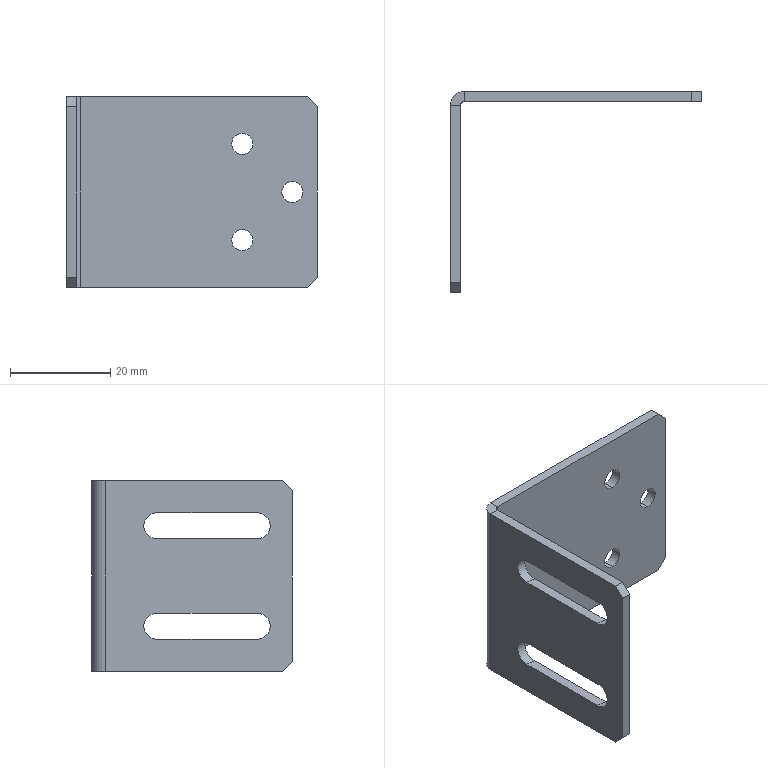Part | SolidWorks | features Chamfer 1, Cut 1, FlatPattern 1, HoleWzd 1, SMBaseFlange 1, SheetMetal 1 | 1 solid | 32 faces | box 50 x 40 x 38 mm | volume 6031 mm3 | plane 20 | cylinder 12 | commonest cylinder face diameters 4.2 x6 5.2 x4 1.473 x1 5.473 x1
STEP:
#1=CARTESIAN_POINT('',(35.,38.,7.5));
#2=VERTEX_POINT('',#1);
#3=CARTESIAN_POINT('',(35.,38.,11.7));
#4=VERTEX_POINT('',#3);
#5=CARTESIAN_POINT('',(35.,38.,9.6));
#6=DIRECTION('',(0.,1.,0.));
#7=DIRECTION('',(0.,0.,1.));
#8=AXIS2_PLACEMENT_3D('',#5,#6,#7);
#9=CIRCLE('',#8,2.1);
#10=EDGE_CURVE('',#2,#4,#9,.T.);
#11=ORIENTED_EDGE('',*,*,#10,.F.);
#12=CARTESIAN_POINT('',(35.,40.,7.5));
#13=VERTEX_POINT('',#12);
#14=CARTESIAN_POINT('',(35.,40.,7.5));
#15=DIRECTION('',(0.,1.,0.));
#16=VECTOR('',#15,1000.);
#17=LINE('',#14,#16);
#18=EDGE_CURVE('',#2,#13,#17,.T.);
#19=ORIENTED_EDGE('',*,*,#18,.T.);
#20=CARTESIAN_POINT('',(35.,40.,11.7));
#21=VERTEX_POINT('',#20);
#22=CARTESIAN_POINT('',(35.,40.,9.6));
#23=DIRECTION('',(0.,1.,0.));
#24=DIRECTION('',(0.,0.,1.));
#25=AXIS2_PLACEMENT_3D('',#22,#23,#24);
#26=CIRCLE('',#25,2.1);
#27=EDGE_CURVE('',#13,#21,#26,.T.);
#28=ORIENTED_EDGE('',*,*,#27,.T.);
#29=CARTESIAN_POINT('',(35.,40.,11.7));
#30=DIRECTION('',(0.,1.,0.));
#31=VECTOR('',#30,1000.);
#32=LINE('',#29,#31);
#33=EDGE_CURVE('',#4,#21,#32,.T.);
#34=ORIENTED_EDGE('',*,*,#33,.F.);
#35=EDGE_LOOP('',(#11,#19,#28,#34));
#36=FACE_OUTER_BOUND('',#35,.T.);
#37=CARTESIAN_POINT('',(35.,40.,9.6));
#38=DIRECTION('',(0.,1.,0.));
#39=DIRECTION('',(0.,0.,1.));
#40=AXIS2_PLACEMENT_3D('',#37,#38,#39);
#41=CYLINDRICAL_SURFACE('',#40,2.1);
#42=ADVANCED_FACE('',(#36),#41,.F.);
#43=CARTESIAN_POINT('',(45.,38.,-2.1));
#44=VERTEX_POINT('',#43);
#45=CARTESIAN_POINT('',(45.,38.,2.1));
#46=VERTEX_POINT('',#45);
#47=CARTESIAN_POINT('',(45.,38.,0.));
#48=DIRECTION('',(0.,1.,0.));
#49=DIRECTION('',(0.,0.,1.));
#50=AXIS2_PLACEMENT_3D('',#47,#48,#49);
#51=CIRCLE('',#50,2.1);
#52=EDGE_CURVE('',#44,#46,#51,.T.);
#53=ORIENTED_EDGE('',*,*,#52,.F.);
#54=CARTESIAN_POINT('',(45.,40.,-2.1));
#55=VERTEX_POINT('',#54);
#56=CARTESIAN_POINT('',(45.,40.,-2.1));
#57=DIRECTION('',(0.,1.,0.));
#58=VECTOR('',#57,1000.);
#59=LINE('',#56,#58);
#60=EDGE_CURVE('',#44,#55,#59,.T.);
#61=ORIENTED_EDGE('',*,*,#60,.T.);
#62=CARTESIAN_POINT('',(45.,40.,2.1));
#63=VERTEX_POINT('',#62);
#64=CARTESIAN_POINT('',(45.,40.,0.));
#65=DIRECTION('',(0.,1.,0.));
#66=DIRECTION('',(0.,0.,1.));
#67=AXIS2_PLACEMENT_3D('',#64,#65,#66);
#68=CIRCLE('',#67,2.1);
#69=EDGE_CURVE('',#55,#63,#68,.T.);
#70=ORIENTED_EDGE('',*,*,#69,.T.);
#71=CARTESIAN_POINT('',(45.,40.,2.1));
#72=DIRECTION('',(0.,1.,0.));
#73=VECTOR('',#72,1000.);
#74=LINE('',#71,#73);
#75=EDGE_CURVE('',#46,#63,#74,.T.);
#76=ORIENTED_EDGE('',*,*,#75,.F.);
#77=EDGE_LOOP('',(#53,#61,#70,#76));
#78=FACE_OUTER_BOUND('',#77,.T.);
#79=CARTESIAN_POINT('',(45.,40.,0.));
#80=DIRECTION('',(0.,1.,0.));
#81=DIRECTION('',(0.,0.,1.));
#82=AXIS2_PLACEMENT_3D('',#79,#80,#81);
#83=CYLINDRICAL_SURFACE('',#82,2.1);
#84=ADVANCED_FACE('',(#78),#83,.F.);
#85=CARTESIAN_POINT('',(35.,38.,-11.7));
#86=VERTEX_POINT('',#85);
#87=CARTESIAN_POINT('',(35.,38.,-7.5));
#88=VERTEX_POINT('',#87);
#89=CARTESIAN_POINT('',(35.,38.,-9.6));
#90=DIRECTION('',(0.,1.,0.));
#91=DIRECTION('',(0.,0.,1.));
#92=AXIS2_PLACEMENT_3D('',#89,#90,#91);
#93=CIRCLE('',#92,2.1);
#94=EDGE_CURVE('',#86,#88,#93,.T.);
#95=ORIENTED_EDGE('',*,*,#94,.F.);
#96=CARTESIAN_POINT('',(35.,40.,-11.7));
#97=VERTEX_POINT('',#96);
#98=CARTESIAN_POINT('',(35.,40.,-11.7));
#99=DIRECTION('',(0.,1.,0.));
#100=VECTOR('',#99,1000.);
#101=LINE('',#98,#100);
#102=EDGE_CURVE('',#86,#97,#101,.T.);
#103=ORIENTED_EDGE('',*,*,#102,.T.);
#104=CARTESIAN_POINT('',(35.,40.,-7.5));
#105=VERTEX_POINT('',#104);
#106=CARTESIAN_POINT('',(35.,40.,-9.6));
#107=DIRECTION('',(0.,1.,0.));
#108=DIRECTION('',(0.,0.,1.));
#109=AXIS2_PLACEMENT_3D('',#106,#107,#108);
#110=CIRCLE('',#109,2.1);
#111=EDGE_CURVE('',#97,#105,#110,.T.);
#112=ORIENTED_EDGE('',*,*,#111,.T.);
#113=CARTESIAN_POINT('',(35.,40.,-7.5));
#114=DIRECTION('',(0.,1.,0.));
#115=VECTOR('',#114,1000.);
#116=LINE('',#113,#115);
#117=EDGE_CURVE('',#88,#105,#116,.T.);
#118=ORIENTED_EDGE('',*,*,#117,.F.);
#119=EDGE_LOOP('',(#95,#103,#112,#118));
#120=FACE_OUTER_BOUND('',#119,.T.);
#121=CARTESIAN_POINT('',(35.,40.,-9.6));
#122=DIRECTION('',(0.,1.,0.));
#123=DIRECTION('',(0.,0.,1.));
#124=AXIS2_PLACEMENT_3D('',#121,#122,#123);
#125=CYLINDRICAL_SURFACE('',#124,2.1);
#126=ADVANCED_FACE('',(#120),#125,.F.);
#127=CARTESIAN_POINT('',(2.737,40.,19.));
#128=VERTEX_POINT('',#127);
#129=CARTESIAN_POINT('',(2.737,38.,19.));
#130=VERTEX_POINT('',#129);
#131=CARTESIAN_POINT('',(2.737,40.,19.));
#132=DIRECTION('',(0.,-1.,0.));
#133=VECTOR('',#132,1000.);
#134=LINE('',#131,#133);
#135=EDGE_CURVE('',#128,#130,#134,.T.);
#136=ORIENTED_EDGE('',*,*,#135,.F.);
#137=CARTESIAN_POINT('',(0.,37.263,19.));
#138=VERTEX_POINT('',#137);
#139=CARTESIAN_POINT('',(2.737,37.263,19.));
#140=DIRECTION('',(0.,0.,-1.));
#141=DIRECTION('',(1.,0.,0.));
#142=AXIS2_PLACEMENT_3D('',#139,#140,#141);
#143=CIRCLE('',#142,2.737);
#144=EDGE_CURVE('',#138,#128,#143,.T.);
#145=ORIENTED_EDGE('',*,*,#144,.F.);
#146=CARTESIAN_POINT('',(2.,37.263,19.));
#147=VERTEX_POINT('',#146);
#148=CARTESIAN_POINT('',(2.,37.263,19.));
#149=DIRECTION('',(-1.,0.,0.));
#150=VECTOR('',#149,1000.);
#151=LINE('',#148,#150);
#152=EDGE_CURVE('',#147,#138,#151,.T.);
#153=ORIENTED_EDGE('',*,*,#152,.F.);
#154=CARTESIAN_POINT('',(2.737,37.263,19.));
#155=DIRECTION('',(0.,0.,-1.));
#156=DIRECTION('',(1.,0.,0.));
#157=AXIS2_PLACEMENT_3D('',#154,#155,#156);
#158=CIRCLE('',#157,0.7366);
#159=EDGE_CURVE('',#147,#130,#158,.T.);
#160=ORIENTED_EDGE('',*,*,#159,.T.);
#161=EDGE_LOOP('',(#136,#145,#153,#160));
#162=FACE_OUTER_BOUND('',#161,.T.);
#163=CARTESIAN_POINT('',(2.737,40.,19.));
#164=DIRECTION('',(0.,0.,1.));
#165=DIRECTION('',(1.,0.,0.));
#166=AXIS2_PLACEMENT_3D('',#163,#164,#165);
#167=PLANE('',#166);
#168=ADVANCED_FACE('',(#162),#167,.T.);
#169=CARTESIAN_POINT('',(48.,38.,19.));
#170=VERTEX_POINT('',#169);
#171=CARTESIAN_POINT('',(0.,38.,19.));
#172=DIRECTION('',(1.,0.,0.));
#173=VECTOR('',#172,1000.);
#174=LINE('',#171,#173);
#175=EDGE_CURVE('',#130,#170,#174,.T.);
#176=ORIENTED_EDGE('',*,*,#175,.T.);
#177=CARTESIAN_POINT('',(48.,40.,19.));
#178=VERTEX_POINT('',#177);
#179=CARTESIAN_POINT('',(48.,37.263,19.));
#180=DIRECTION('',(0.,1.,0.));
#181=VECTOR('',#180,1000.);
#182=LINE('',#179,#181);
#183=EDGE_CURVE('',#170,#178,#182,.T.);
#184=ORIENTED_EDGE('',*,*,#183,.T.);
#185=CARTESIAN_POINT('',(0.,40.,19.));
#186=DIRECTION('',(1.,0.,0.));
#187=VECTOR('',#186,1000.);
#188=LINE('',#185,#187);
#189=EDGE_CURVE('',#128,#178,#188,.T.);
#190=ORIENTED_EDGE('',*,*,#189,.F.);
#191=ORIENTED_EDGE('',*,*,#135,.T.);
#192=EDGE_LOOP('',(#176,#184,#190,#191));
#193=FACE_OUTER_BOUND('',#192,.T.);
#194=CARTESIAN_POINT('',(2.,37.263,19.));
#195=DIRECTION('',(0.,0.,1.));
#196=DIRECTION('',(1.,0.,0.));
#197=AXIS2_PLACEMENT_3D('',#194,#195,#196);
#198=PLANE('',#197);
#199=ADVANCED_FACE('',(#193),#198,.T.);
#200=CARTESIAN_POINT('',(0.,37.263,-19.));
#201=VERTEX_POINT('',#200);
#202=CARTESIAN_POINT('',(2.,37.263,-19.));
#203=VERTEX_POINT('',#202);
#204=CARTESIAN_POINT('',(0.,37.263,-19.));
#205=DIRECTION('',(1.,0.,0.));
#206=VECTOR('',#205,1000.);
#207=LINE('',#204,#206);
#208=EDGE_CURVE('',#201,#203,#207,.T.);
#209=ORIENTED_EDGE('',*,*,#208,.F.);
#210=CARTESIAN_POINT('',(2.737,40.,-19.));
#211=VERTEX_POINT('',#210);
#212=CARTESIAN_POINT('',(2.737,37.263,-19.));
#213=DIRECTION('',(0.,0.,-1.));
#214=DIRECTION('',(1.,0.,0.));
#215=AXIS2_PLACEMENT_3D('',#212,#213,#214);
#216=CIRCLE('',#215,2.737);
#217=EDGE_CURVE('',#201,#211,#216,.T.);
#218=ORIENTED_EDGE('',*,*,#217,.T.);
#219=CARTESIAN_POINT('',(2.737,38.,-19.));
#220=VERTEX_POINT('',#219);
#221=CARTESIAN_POINT('',(2.737,38.,-19.));
#222=DIRECTION('',(0.,1.,0.));
#223=VECTOR('',#222,1000.);
#224=LINE('',#221,#223);
#225=EDGE_CURVE('',#220,#211,#224,.T.);
#226=ORIENTED_EDGE('',*,*,#225,.F.);
#227=CARTESIAN_POINT('',(2.737,37.263,-19.));
#228=DIRECTION('',(0.,0.,-1.));
#229=DIRECTION('',(1.,0.,0.));
#230=AXIS2_PLACEMENT_3D('',#227,#228,#229);
#231=CIRCLE('',#230,0.7366);
#232=EDGE_CURVE('',#203,#220,#231,.T.);
#233=ORIENTED_EDGE('',*,*,#232,.F.);
#234=EDGE_LOOP('',(#209,#218,#226,#233));
#235=FACE_OUTER_BOUND('',#234,.T.);
#236=CARTESIAN_POINT('',(0.,37.263,-19.));
#237=DIRECTION('',(0.,0.,-1.));
#238=DIRECTION('',(-1.,0.,0.));
#239=AXIS2_PLACEMENT_3D('',#236,#237,#238);
#240=PLANE('',#239);
#241=ADVANCED_FACE('',(#235),#240,.T.);
#242=CARTESIAN_POINT('',(2.,2.,-19.));
#243=VERTEX_POINT('',#242);
#244=CARTESIAN_POINT('',(2.,0.,-19.));
#245=DIRECTION('',(0.,1.,0.));
#246=VECTOR('',#245,1000.);
#247=LINE('',#244,#246);
#248=EDGE_CURVE('',#243,#203,#247,.T.);
#249=ORIENTED_EDGE('',*,*,#248,.F.);
#250=CARTESIAN_POINT('',(0.,2.,-19.));
#251=VERTEX_POINT('',#250);
#252=CARTESIAN_POINT('',(2.737,2.,-19.));
#253=DIRECTION('',(-1.,0.,0.));
#254=VECTOR('',#253,1000.);
#255=LINE('',#252,#254);
#256=EDGE_CURVE('',#243,#251,#255,.T.);
#257=ORIENTED_EDGE('',*,*,#256,.T.);
#258=CARTESIAN_POINT('',(0.,0.,-19.));
#259=DIRECTION('',(0.,1.,0.));
#260=VECTOR('',#259,1000.);
#261=LINE('',#258,#260);
#262=EDGE_CURVE('',#251,#201,#261,.T.);
#263=ORIENTED_EDGE('',*,*,#262,.T.);
#264=ORIENTED_EDGE('',*,*,#208,.T.);
#265=EDGE_LOOP('',(#249,#257,#263,#264));
#266=FACE_OUTER_BOUND('',#265,.T.);
#267=CARTESIAN_POINT('',(2.737,38.,-19.));
#268=DIRECTION('',(0.,0.,-1.));
#269=DIRECTION('',(-1.,0.,0.));
#270=AXIS2_PLACEMENT_3D('',#267,#268,#269);
#271=PLANE('',#270);
#272=ADVANCED_FACE('',(#266),#271,.T.);
#273=CARTESIAN_POINT('',(35.,38.,9.6));
#274=DIRECTION('',(0.,1.,0.));
#275=DIRECTION('',(0.,0.,1.));
#276=AXIS2_PLACEMENT_3D('',#273,#274,#275);
#277=CIRCLE('',#276,2.1);
#278=EDGE_CURVE('',#4,#2,#277,.T.);
#279=ORIENTED_EDGE('',*,*,#278,.T.);
#280=ORIENTED_EDGE('',*,*,#10,.T.);
#281=EDGE_LOOP('',(#279,#280));
#282=FACE_BOUND('',#281,.T.);
#283=CARTESIAN_POINT('',(45.,38.,0.));
#284=DIRECTION('',(0.,1.,0.));
#285=DIRECTION('',(0.,0.,1.));
#286=AXIS2_PLACEMENT_3D('',#283,#284,#285);
#287=CIRCLE('',#286,2.1);
#288=EDGE_CURVE('',#46,#44,#287,.T.);
#289=ORIENTED_EDGE('',*,*,#288,.T.);
#290=ORIENTED_EDGE('',*,*,#52,.T.);
#291=EDGE_LOOP('',(#289,#290));
#292=FACE_BOUND('',#291,.T.);
#293=CARTESIAN_POINT('',(35.,38.,-9.6));
#294=DIRECTION('',(0.,1.,0.));
#295=DIRECTION('',(0.,0.,1.));
#296=AXIS2_PLACEMENT_3D('',#293,#294,#295);
#297=CIRCLE('',#296,2.1);
#298=EDGE_CURVE('',#88,#86,#297,.T.);
#299=ORIENTED_EDGE('',*,*,#298,.T.);
#300=ORIENTED_EDGE('',*,*,#94,.T.);
#301=EDGE_LOOP('',(#299,#300));
#302=FACE_BOUND('',#301,.T.);
#303=CARTESIAN_POINT('',(48.,38.,-19.));
#304=VERTEX_POINT('',#303);
#305=CARTESIAN_POINT('',(0.,38.,-19.));
#306=DIRECTION('',(1.,0.,0.));
#307=VECTOR('',#306,1000.);
#308=LINE('',#305,#307);
#309=EDGE_CURVE('',#220,#304,#308,.T.);
#310=ORIENTED_EDGE('',*,*,#309,.T.);
#311=CARTESIAN_POINT('',(50.,38.,-17.));
#312=VERTEX_POINT('',#311);
#313=CARTESIAN_POINT('',(48.,38.,-19.));
#314=DIRECTION('',(0.7071,0.,0.7071));
#315=VECTOR('',#314,1000.);
#316=LINE('',#313,#315);
#317=EDGE_CURVE('',#304,#312,#316,.T.);
#318=ORIENTED_EDGE('',*,*,#317,.T.);
#319=CARTESIAN_POINT('',(50.,38.,17.));
#320=VERTEX_POINT('',#319);
#321=CARTESIAN_POINT('',(50.,38.,19.));
#322=DIRECTION('',(0.,0.,-1.));
#323=VECTOR('',#322,1000.);
#324=LINE('',#321,#323);
#325=EDGE_CURVE('',#320,#312,#324,.T.);
#326=ORIENTED_EDGE('',*,*,#325,.F.);
#327=CARTESIAN_POINT('',(50.,38.,17.));
#328=DIRECTION('',(-0.7071,0.,0.7071));
#329=VECTOR('',#328,1000.);
#330=LINE('',#327,#329);
#331=EDGE_CURVE('',#320,#170,#330,.T.);
#332=ORIENTED_EDGE('',*,*,#331,.T.);
#333=ORIENTED_EDGE('',*,*,#175,.F.);
#334=CARTESIAN_POINT('',(2.737,38.,19.));
#335=DIRECTION('',(0.,0.,-1.));
#336=VECTOR('',#335,1000.);
#337=LINE('',#334,#336);
#338=EDGE_CURVE('',#130,#220,#337,.T.);
#339=ORIENTED_EDGE('',*,*,#338,.T.);
#340=EDGE_LOOP('',(#310,#318,#326,#332,#333,#339));
#341=FACE_OUTER_BOUND('',#340,.T.);
#342=CARTESIAN_POINT('',(0.,38.,19.));
#343=DIRECTION('',(0.,1.,0.));
#344=DIRECTION('',(0.,0.,1.));
#345=AXIS2_PLACEMENT_3D('',#342,#343,#344);
#346=PLANE('',#345);
#347=ADVANCED_FACE('',(#282,#292,#302,#341),#346,.F.);
#348=ORIENTED_EDGE('',*,*,#325,.T.);
#349=CARTESIAN_POINT('',(50.,40.,-17.));
#350=VERTEX_POINT('',#349);
#351=CARTESIAN_POINT('',(50.,40.,-17.));
#352=DIRECTION('',(0.,1.,0.));
#353=VECTOR('',#352,1000.);
#354=LINE('',#351,#353);
#355=EDGE_CURVE('',#312,#350,#354,.T.);
#356=ORIENTED_EDGE('',*,*,#355,.T.);
#357=CARTESIAN_POINT('',(50.,40.,17.));
#358=VERTEX_POINT('',#357);
#359=CARTESIAN_POINT('',(50.,40.,19.));
#360=DIRECTION('',(0.,0.,-1.));
#361=VECTOR('',#360,1000.);
#362=LINE('',#359,#361);
#363=EDGE_CURVE('',#358,#350,#362,.T.);
#364=ORIENTED_EDGE('',*,*,#363,.F.);
#365=CARTESIAN_POINT('',(50.,40.,17.));
#366=DIRECTION('',(0.,-1.,0.));
#367=VECTOR('',#366,1000.);
#368=LINE('',#365,#367);
#369=EDGE_CURVE('',#358,#320,#368,.T.);
#370=ORIENTED_EDGE('',*,*,#369,.T.);
#371=EDGE_LOOP('',(#348,#356,#364,#370));
#372=FACE_OUTER_BOUND('',#371,.T.);
#373=CARTESIAN_POINT('',(50.,40.,19.));
#374=DIRECTION('',(1.,0.,0.));
#375=DIRECTION('',(0.,0.,-1.));
#376=AXIS2_PLACEMENT_3D('',#373,#374,#375);
#377=PLANE('',#376);
#378=ADVANCED_FACE('',(#372),#377,.T.);
#379=CARTESIAN_POINT('',(35.,40.,9.6));
#380=DIRECTION('',(0.,1.,0.));
#381=DIRECTION('',(0.,0.,1.));
#382=AXIS2_PLACEMENT_3D('',#379,#380,#381);
#383=CIRCLE('',#382,2.1);
#384=EDGE_CURVE('',#21,#13,#383,.T.);
#385=ORIENTED_EDGE('',*,*,#384,.F.);
#386=ORIENTED_EDGE('',*,*,#27,.F.);
#387=EDGE_LOOP('',(#385,#386));
#388=FACE_BOUND('',#387,.T.);
#389=CARTESIAN_POINT('',(45.,40.,0.));
#390=DIRECTION('',(0.,1.,0.));
#391=DIRECTION('',(0.,0.,1.));
#392=AXIS2_PLACEMENT_3D('',#389,#390,#391);
#393=CIRCLE('',#392,2.1);
#394=EDGE_CURVE('',#63,#55,#393,.T.);
#395=ORIENTED_EDGE('',*,*,#394,.F.);
#396=ORIENTED_EDGE('',*,*,#69,.F.);
#397=EDGE_LOOP('',(#395,#396));
#398=FACE_BOUND('',#397,.T.);
#399=CARTESIAN_POINT('',(35.,40.,-9.6));
#400=DIRECTION('',(0.,1.,0.));
#401=DIRECTION('',(0.,0.,1.));
#402=AXIS2_PLACEMENT_3D('',#399,#400,#401);
#403=CIRCLE('',#402,2.1);
#404=EDGE_CURVE('',#105,#97,#403,.T.);
#405=ORIENTED_EDGE('',*,*,#404,.F.);
#406=ORIENTED_EDGE('',*,*,#111,.F.);
#407=EDGE_LOOP('',(#405,#406));
#408=FACE_BOUND('',#407,.T.);
#409=ORIENTED_EDGE('',*,*,#363,.T.);
#410=CARTESIAN_POINT('',(48.,40.,-19.));
#411=VERTEX_POINT('',#410);
#412=CARTESIAN_POINT('',(43.,40.,-24.));
#413=DIRECTION('',(-0.7071,0.,-0.7071));
#414=VECTOR('',#413,1000.);
#415=LINE('',#412,#414);
#416=EDGE_CURVE('',#350,#411,#415,.T.);
#417=ORIENTED_EDGE('',*,*,#416,.T.);
#418=CARTESIAN_POINT('',(0.,40.,-19.));
#419=DIRECTION('',(1.,0.,0.));
#420=VECTOR('',#419,1000.);
#421=LINE('',#418,#420);
#422=EDGE_CURVE('',#211,#411,#421,.T.);
#423=ORIENTED_EDGE('',*,*,#422,.F.);
#424=CARTESIAN_POINT('',(2.737,40.,19.));
#425=DIRECTION('',(0.,0.,-1.));
#426=VECTOR('',#425,1000.);
#427=LINE('',#424,#426);
#428=EDGE_CURVE('',#128,#211,#427,.T.);
#429=ORIENTED_EDGE('',*,*,#428,.F.);
#430=ORIENTED_EDGE('',*,*,#189,.T.);
#431=CARTESIAN_POINT('',(24.,40.,43.));
#432=DIRECTION('',(0.7071,0.,-0.7071));
#433=VECTOR('',#432,1000.);
#434=LINE('',#431,#433);
#435=EDGE_CURVE('',#178,#358,#434,.T.);
#436=ORIENTED_EDGE('',*,*,#435,.T.);
#437=EDGE_LOOP('',(#409,#417,#423,#429,#430,#436));
#438=FACE_OUTER_BOUND('',#437,.T.);
#439=CARTESIAN_POINT('',(0.,40.,19.));
#440=DIRECTION('',(0.,1.,0.));
#441=DIRECTION('',(0.,0.,1.));
#442=AXIS2_PLACEMENT_3D('',#439,#440,#441);
#443=PLANE('',#442);
#444=ADVANCED_FACE('',(#388,#398,#408,#438),#443,.T.);
#445=ORIENTED_EDGE('',*,*,#217,.F.);
#446=CARTESIAN_POINT('',(0.,37.263,19.));
#447=DIRECTION('',(0.,0.,-1.));
#448=VECTOR('',#447,1000.);
#449=LINE('',#446,#448);
#450=EDGE_CURVE('',#138,#201,#449,.T.);
#451=ORIENTED_EDGE('',*,*,#450,.F.);
#452=ORIENTED_EDGE('',*,*,#144,.T.);
#453=ORIENTED_EDGE('',*,*,#428,.T.);
#454=EDGE_LOOP('',(#445,#451,#452,#453));
#455=FACE_OUTER_BOUND('',#454,.T.);
#456=CARTESIAN_POINT('',(2.737,37.263,19.));
#457=DIRECTION('',(0.,0.,-1.));
#458=DIRECTION('',(-1.,0.,0.));
#459=AXIS2_PLACEMENT_3D('',#456,#457,#458);
#460=CYLINDRICAL_SURFACE('',#459,2.737);
#461=ADVANCED_FACE('',(#455),#460,.T.);
#462=CARTESIAN_POINT('',(0.,7.,7.4));
#463=VERTEX_POINT('',#462);
#464=CARTESIAN_POINT('',(0.,7.,12.6));
#465=VERTEX_POINT('',#464);
#466=CARTESIAN_POINT('',(0.,7.,10.));
#467=DIRECTION('',(-1.,0.,0.));
#468=DIRECTION('',(0.,0.,-1.));
#469=AXIS2_PLACEMENT_3D('',#466,#467,#468);
#470=CIRCLE('',#469,2.6);
#471=EDGE_CURVE('',#463,#465,#470,.T.);
#472=ORIENTED_EDGE('',*,*,#471,.F.);
#473=CARTESIAN_POINT('',(0.,27.,7.4));
#474=VERTEX_POINT('',#473);
#475=CARTESIAN_POINT('',(0.,27.,7.4));
#476=DIRECTION('',(0.,-1.,0.));
#477=VECTOR('',#476,1000.);
#478=LINE('',#475,#477);
#479=EDGE_CURVE('',#474,#463,#478,.T.);
#480=ORIENTED_EDGE('',*,*,#479,.F.);
#481=CARTESIAN_POINT('',(0.,27.,12.6));
#482=VERTEX_POINT('',#481);
#483=CARTESIAN_POINT('',(0.,27.,10.));
#484=DIRECTION('',(-1.,0.,0.));
#485=DIRECTION('',(0.,0.,1.));
#486=AXIS2_PLACEMENT_3D('',#483,#484,#485);
#487=CIRCLE('',#486,2.6);
#488=EDGE_CURVE('',#482,#474,#487,.T.);
#489=ORIENTED_EDGE('',*,*,#488,.F.);
#490=CARTESIAN_POINT('',(0.,27.,12.6));
#491=DIRECTION('',(0.,1.,0.));
#492=VECTOR('',#491,1000.);
#493=LINE('',#490,#492);
#494=EDGE_CURVE('',#465,#482,#493,.T.);
#495=ORIENTED_EDGE('',*,*,#494,.F.);
#496=EDGE_LOOP('',(#472,#480,#489,#495));
#497=FACE_BOUND('',#496,.T.);
#498=CARTESIAN_POINT('',(0.,27.,-7.4));
#499=VERTEX_POINT('',#498);
#500=CARTESIAN_POINT('',(0.,27.,-12.6));
#501=VERTEX_POINT('',#500);
#502=CARTESIAN_POINT('',(0.,27.,-10.));
#503=DIRECTION('',(-1.,0.,0.));
#504=DIRECTION('',(0.,0.,-1.));
#505=AXIS2_PLACEMENT_3D('',#502,#503,#504);
#506=CIRCLE('',#505,2.6);
#507=EDGE_CURVE('',#499,#501,#506,.T.);
#508=ORIENTED_EDGE('',*,*,#507,.F.);
#509=CARTESIAN_POINT('',(0.,7.,-7.4));
#510=VERTEX_POINT('',#509);
#511=CARTESIAN_POINT('',(0.,27.,-7.4));
#512=DIRECTION('',(0.,1.,0.));
#513=VECTOR('',#512,1000.);
#514=LINE('',#511,#513);
#515=EDGE_CURVE('',#510,#499,#514,.T.);
#516=ORIENTED_EDGE('',*,*,#515,.F.);
#517=CARTESIAN_POINT('',(0.,7.,-12.6));
#518=VERTEX_POINT('',#517);
#519=CARTESIAN_POINT('',(0.,7.,-10.));
#520=DIRECTION('',(-1.,0.,0.));
#521=DIRECTION('',(0.,0.,1.));
#522=AXIS2_PLACEMENT_3D('',#519,#520,#521);
#523=CIRCLE('',#522,2.6);
#524=EDGE_CURVE('',#518,#510,#523,.T.);
#525=ORIENTED_EDGE('',*,*,#524,.F.);
#526=CARTESIAN_POINT('',(0.,27.,-12.6));
#527=DIRECTION('',(0.,-1.,0.));
#528=VECTOR('',#527,1000.);
#529=LINE('',#526,#528);
#530=EDGE_CURVE('',#501,#518,#529,.T.);
#531=ORIENTED_EDGE('',*,*,#530,.F.);
#532=EDGE_LOOP('',(#508,#516,#525,#531));
#533=FACE_BOUND('',#532,.T.);
#534=ORIENTED_EDGE('',*,*,#262,.F.);
#535=CARTESIAN_POINT('',(0.,0.,-17.));
#536=VERTEX_POINT('',#535);
#537=CARTESIAN_POINT('',(0.,-18.,1.));
#538=DIRECTION('',(0.,-0.7071,0.7071));
#539=VECTOR('',#538,1000.);
#540=LINE('',#537,#539);
#541=EDGE_CURVE('',#251,#536,#540,.T.);
#542=ORIENTED_EDGE('',*,*,#541,.T.);
#543=CARTESIAN_POINT('',(0.,0.,17.));
#544=VERTEX_POINT('',#543);
#545=CARTESIAN_POINT('',(0.,0.,19.));
#546=DIRECTION('',(0.,0.,-1.));
#547=VECTOR('',#546,1000.);
#548=LINE('',#545,#547);
#549=EDGE_CURVE('',#544,#536,#548,.T.);
#550=ORIENTED_EDGE('',*,*,#549,.F.);
#551=CARTESIAN_POINT('',(0.,2.,19.));
#552=VERTEX_POINT('',#551);
#553=CARTESIAN_POINT('',(0.,1.,18.));
#554=DIRECTION('',(0.,0.7071,0.7071));
#555=VECTOR('',#554,1000.);
#556=LINE('',#553,#555);
#557=EDGE_CURVE('',#544,#552,#556,.T.);
#558=ORIENTED_EDGE('',*,*,#557,.T.);
#559=CARTESIAN_POINT('',(0.,0.,19.));
#560=DIRECTION('',(0.,1.,0.));
#561=VECTOR('',#560,1000.);
#562=LINE('',#559,#561);
#563=EDGE_CURVE('',#552,#138,#562,.T.);
#564=ORIENTED_EDGE('',*,*,#563,.T.);
#565=ORIENTED_EDGE('',*,*,#450,.T.);
#566=EDGE_LOOP('',(#534,#542,#550,#558,#564,#565));
#567=FACE_OUTER_BOUND('',#566,.T.);
#568=CARTESIAN_POINT('',(0.,0.,19.));
#569=DIRECTION('',(-1.,0.,0.));
#570=DIRECTION('',(0.,0.,1.));
#571=AXIS2_PLACEMENT_3D('',#568,#569,#570);
#572=PLANE('',#571);
#573=ADVANCED_FACE('',(#497,#533,#567),#572,.T.);
#574=ORIENTED_EDGE('',*,*,#549,.T.);
#575=CARTESIAN_POINT('',(2.,0.,-17.));
#576=VERTEX_POINT('',#575);
#577=CARTESIAN_POINT('',(2.,0.,-17.));
#578=DIRECTION('',(1.,0.,0.));
#579=VECTOR('',#578,1000.);
#580=LINE('',#577,#579);
#581=EDGE_CURVE('',#536,#576,#580,.T.);
#582=ORIENTED_EDGE('',*,*,#581,.T.);
#583=CARTESIAN_POINT('',(2.,0.,17.));
#584=VERTEX_POINT('',#583);
#585=CARTESIAN_POINT('',(2.,0.,19.));
#586=DIRECTION('',(0.,0.,-1.));
#587=VECTOR('',#586,1000.);
#588=LINE('',#585,#587);
#589=EDGE_CURVE('',#584,#576,#588,.T.);
#590=ORIENTED_EDGE('',*,*,#589,.F.);
#591=CARTESIAN_POINT('',(2.,0.,17.));
#592=DIRECTION('',(-1.,0.,0.));
#593=VECTOR('',#592,1000.);
#594=LINE('',#591,#593);
#595=EDGE_CURVE('',#584,#544,#594,.T.);
#596=ORIENTED_EDGE('',*,*,#595,.T.);
#597=EDGE_LOOP('',(#574,#582,#590,#596));
#598=FACE_OUTER_BOUND('',#597,.T.);
#599=CARTESIAN_POINT('',(2.,0.,19.));
#600=DIRECTION('',(0.,-1.,0.));
#601=DIRECTION('',(0.,0.,-1.));
#602=AXIS2_PLACEMENT_3D('',#599,#600,#601);
#603=PLANE('',#602);
#604=ADVANCED_FACE('',(#598),#603,.T.);
#605=CARTESIAN_POINT('',(2.,27.,7.4));
#606=VERTEX_POINT('',#605);
#607=CARTESIAN_POINT('',(2.,7.,7.4));
#608=VERTEX_POINT('',#607);
#609=CARTESIAN_POINT('',(2.,0.,7.4));
#610=DIRECTION('',(0.,-1.,0.));
#611=VECTOR('',#610,1000.);
#612=LINE('',#609,#611);
#613=EDGE_CURVE('',#606,#608,#612,.T.);
#614=ORIENTED_EDGE('',*,*,#613,.T.);
#615=CARTESIAN_POINT('',(2.,7.,12.6));
#616=VERTEX_POINT('',#615);
#617=CARTESIAN_POINT('',(2.,7.,10.));
#618=DIRECTION('',(-1.,0.,0.));
#619=DIRECTION('',(0.,0.,1.));
#620=AXIS2_PLACEMENT_3D('',#617,#618,#619);
#621=CIRCLE('',#620,2.6);
#622=EDGE_CURVE('',#608,#616,#621,.T.);
#623=ORIENTED_EDGE('',*,*,#622,.T.);
#624=CARTESIAN_POINT('',(2.,27.,12.6));
#625=VERTEX_POINT('',#624);
#626=CARTESIAN_POINT('',(2.,0.,12.6));
#627=DIRECTION('',(0.,1.,0.));
#628=VECTOR('',#627,1000.);
#629=LINE('',#626,#628);
#630=EDGE_CURVE('',#616,#625,#629,.T.);
#631=ORIENTED_EDGE('',*,*,#630,.T.);
#632=CARTESIAN_POINT('',(2.,27.,10.));
#633=DIRECTION('',(-1.,0.,0.));
#634=DIRECTION('',(0.,0.,1.));
#635=AXIS2_PLACEMENT_3D('',#632,#633,#634);
#636=CIRCLE('',#635,2.6);
#637=EDGE_CURVE('',#625,#606,#636,.T.);
#638=ORIENTED_EDGE('',*,*,#637,.T.);
#639=EDGE_LOOP('',(#614,#623,#631,#638));
#640=FACE_BOUND('',#639,.T.);
#641=CARTESIAN_POINT('',(2.,7.,-7.4));
#642=VERTEX_POINT('',#641);
#643=CARTESIAN_POINT('',(2.,27.,-7.4));
#644=VERTEX_POINT('',#643);
#645=CARTESIAN_POINT('',(2.,0.,-7.4));
#646=DIRECTION('',(0.,1.,0.));
#647=VECTOR('',#646,1000.);
#648=LINE('',#645,#647);
#649=EDGE_CURVE('',#642,#644,#648,.T.);
#650=ORIENTED_EDGE('',*,*,#649,.T.);
#651=CARTESIAN_POINT('',(2.,27.,-12.6));
#652=VERTEX_POINT('',#651);
#653=CARTESIAN_POINT('',(2.,27.,-10.));
#654=DIRECTION('',(-1.,0.,0.));
#655=DIRECTION('',(0.,0.,1.));
#656=AXIS2_PLACEMENT_3D('',#653,#654,#655);
#657=CIRCLE('',#656,2.6);
#658=EDGE_CURVE('',#644,#652,#657,.T.);
#659=ORIENTED_EDGE('',*,*,#658,.T.);
#660=CARTESIAN_POINT('',(2.,7.,-12.6));
#661=VERTEX_POINT('',#660);
#662=CARTESIAN_POINT('',(2.,0.,-12.6));
#663=DIRECTION('',(0.,-1.,0.));
#664=VECTOR('',#663,1000.);
#665=LINE('',#662,#664);
#666=EDGE_CURVE('',#652,#661,#665,.T.);
#667=ORIENTED_EDGE('',*,*,#666,.T.);
#668=CARTESIAN_POINT('',(2.,7.,-10.));
#669=DIRECTION('',(-1.,0.,0.));
#670=DIRECTION('',(0.,0.,1.));
#671=AXIS2_PLACEMENT_3D('',#668,#669,#670);
#672=CIRCLE('',#671,2.6);
#673=EDGE_CURVE('',#661,#642,#672,.T.);
#674=ORIENTED_EDGE('',*,*,#673,.T.);
#675=EDGE_LOOP('',(#650,#659,#667,#674));
#676=FACE_BOUND('',#675,.T.);
#677=ORIENTED_EDGE('',*,*,#589,.T.);
#678=CARTESIAN_POINT('',(2.,2.,-19.));
#679=DIRECTION('',(0.,0.7071,-0.7071));
#680=VECTOR('',#679,1000.);
#681=LINE('',#678,#680);
#682=EDGE_CURVE('',#576,#243,#681,.T.);
#683=ORIENTED_EDGE('',*,*,#682,.T.);
#684=ORIENTED_EDGE('',*,*,#248,.T.);
#685=CARTESIAN_POINT('',(2.,37.263,19.));
#686=DIRECTION('',(0.,0.,-1.));
#687=VECTOR('',#686,1000.);
#688=LINE('',#685,#687);
#689=EDGE_CURVE('',#147,#203,#688,.T.);
#690=ORIENTED_EDGE('',*,*,#689,.F.);
#691=CARTESIAN_POINT('',(2.,2.,19.));
#692=VERTEX_POINT('',#691);
#693=CARTESIAN_POINT('',(2.,0.,19.));
#694=DIRECTION('',(0.,1.,0.));
#695=VECTOR('',#694,1000.);
#696=LINE('',#693,#695);
#697=EDGE_CURVE('',#692,#147,#696,.T.);
#698=ORIENTED_EDGE('',*,*,#697,.F.);
#699=CARTESIAN_POINT('',(2.,0.,17.));
#700=DIRECTION('',(0.,-0.7071,-0.7071));
#701=VECTOR('',#700,1000.);
#702=LINE('',#699,#701);
#703=EDGE_CURVE('',#692,#584,#702,.T.);
#704=ORIENTED_EDGE('',*,*,#703,.T.);
#705=EDGE_LOOP('',(#677,#683,#684,#690,#698,#704));
#706=FACE_OUTER_BOUND('',#705,.T.);
#707=CARTESIAN_POINT('',(2.,0.,19.));
#708=DIRECTION('',(-1.,0.,0.));
#709=DIRECTION('',(0.,0.,1.));
#710=AXIS2_PLACEMENT_3D('',#707,#708,#709);
#711=PLANE('',#710);
#712=ADVANCED_FACE('',(#640,#676,#706),#711,.F.);
#713=ORIENTED_EDGE('',*,*,#232,.T.);
#714=ORIENTED_EDGE('',*,*,#338,.F.);
#715=ORIENTED_EDGE('',*,*,#159,.F.);
#716=ORIENTED_EDGE('',*,*,#689,.T.);
#717=EDGE_LOOP('',(#713,#714,#715,#716));
#718=FACE_OUTER_BOUND('',#717,.T.);
#719=CARTESIAN_POINT('',(2.737,37.263,19.));
#720=DIRECTION('',(0.,0.,-1.));
#721=DIRECTION('',(-1.,0.,0.));
#722=AXIS2_PLACEMENT_3D('',#719,#720,#721);
#723=CYLINDRICAL_SURFACE('',#722,0.7366);
#724=ADVANCED_FACE('',(#718),#723,.F.);
#725=ORIENTED_EDGE('',*,*,#563,.F.);
#726=CARTESIAN_POINT('',(2.737,2.,19.));
#727=DIRECTION('',(1.,0.,0.));
#728=VECTOR('',#727,1000.);
#729=LINE('',#726,#728);
#730=EDGE_CURVE('',#552,#692,#729,.T.);
#731=ORIENTED_EDGE('',*,*,#730,.T.);
#732=ORIENTED_EDGE('',*,*,#697,.T.);
#733=ORIENTED_EDGE('',*,*,#152,.T.);
#734=EDGE_LOOP('',(#725,#731,#732,#733));
#735=FACE_OUTER_BOUND('',#734,.T.);
#736=CARTESIAN_POINT('',(2.737,37.263,19.));
#737=DIRECTION('',(0.,0.,1.));
#738=DIRECTION('',(1.,0.,0.));
#739=AXIS2_PLACEMENT_3D('',#736,#737,#738);
#740=PLANE('',#739);
#741=ADVANCED_FACE('',(#735),#740,.T.);
#742=ORIENTED_EDGE('',*,*,#422,.T.);
#743=CARTESIAN_POINT('',(48.,38.,-19.));
#744=DIRECTION('',(0.,-1.,0.));
#745=VECTOR('',#744,1000.);
#746=LINE('',#743,#745);
#747=EDGE_CURVE('',#411,#304,#746,.T.);
#748=ORIENTED_EDGE('',*,*,#747,.T.);
#749=ORIENTED_EDGE('',*,*,#309,.F.);
#750=ORIENTED_EDGE('',*,*,#225,.T.);
#751=EDGE_LOOP('',(#742,#748,#749,#750));
#752=FACE_OUTER_BOUND('',#751,.T.);
#753=CARTESIAN_POINT('',(2.737,37.263,-19.));
#754=DIRECTION('',(0.,0.,1.));
#755=DIRECTION('',(1.,0.,0.));
#756=AXIS2_PLACEMENT_3D('',#753,#754,#755);
#757=PLANE('',#756);
#758=ADVANCED_FACE('',(#752),#757,.F.);
#759=CARTESIAN_POINT('',(50.,27.,-7.4));
#760=DIRECTION('',(-1.,0.,0.));
#761=VECTOR('',#760,1000.);
#762=LINE('',#759,#761);
#763=EDGE_CURVE('',#644,#499,#762,.T.);
#764=ORIENTED_EDGE('',*,*,#763,.T.);
#765=ORIENTED_EDGE('',*,*,#507,.T.);
#766=CARTESIAN_POINT('',(50.,27.,-12.6));
#767=DIRECTION('',(-1.,0.,0.));
#768=VECTOR('',#767,1000.);
#769=LINE('',#766,#768);
#770=EDGE_CURVE('',#652,#501,#769,.T.);
#771=ORIENTED_EDGE('',*,*,#770,.F.);
#772=ORIENTED_EDGE('',*,*,#658,.F.);
#773=EDGE_LOOP('',(#764,#765,#771,#772));
#774=FACE_OUTER_BOUND('',#773,.T.);
#775=CARTESIAN_POINT('',(50.,27.,-10.));
#776=DIRECTION('',(-1.,0.,0.));
#777=DIRECTION('',(0.,0.,1.));
#778=AXIS2_PLACEMENT_3D('',#775,#776,#777);
#779=CYLINDRICAL_SURFACE('',#778,2.6);
#780=ADVANCED_FACE('',(#774),#779,.F.);
#781=CARTESIAN_POINT('',(50.,7.,-7.4));
#782=DIRECTION('',(-1.,0.,0.));
#783=VECTOR('',#782,1000.);
#784=LINE('',#781,#783);
#785=EDGE_CURVE('',#642,#510,#784,.T.);
#786=ORIENTED_EDGE('',*,*,#785,.T.);
#787=ORIENTED_EDGE('',*,*,#515,.T.);
#788=ORIENTED_EDGE('',*,*,#763,.F.);
#789=ORIENTED_EDGE('',*,*,#649,.F.);
#790=EDGE_LOOP('',(#786,#787,#788,#789));
#791=FACE_OUTER_BOUND('',#790,.T.);
#792=CARTESIAN_POINT('',(50.,27.,-7.4));
#793=DIRECTION('',(0.,0.,1.));
#794=DIRECTION('',(0.,-1.,0.));
#795=AXIS2_PLACEMENT_3D('',#792,#793,#794);
#796=PLANE('',#795);
#797=ADVANCED_FACE('',(#791),#796,.F.);
#798=CARTESIAN_POINT('',(50.,7.,-12.6));
#799=DIRECTION('',(-1.,0.,0.));
#800=VECTOR('',#799,1000.);
#801=LINE('',#798,#800);
#802=EDGE_CURVE('',#661,#518,#801,.T.);
#803=ORIENTED_EDGE('',*,*,#802,.T.);
#804=ORIENTED_EDGE('',*,*,#524,.T.);
#805=ORIENTED_EDGE('',*,*,#785,.F.);
#806=ORIENTED_EDGE('',*,*,#673,.F.);
#807=EDGE_LOOP('',(#803,#804,#805,#806));
#808=FACE_OUTER_BOUND('',#807,.T.);
#809=CARTESIAN_POINT('',(50.,7.,-10.));
#810=DIRECTION('',(-1.,0.,0.));
#811=DIRECTION('',(0.,0.,1.));
#812=AXIS2_PLACEMENT_3D('',#809,#810,#811);
#813=CYLINDRICAL_SURFACE('',#812,2.6);
#814=ADVANCED_FACE('',(#808),#813,.F.);
#815=ORIENTED_EDGE('',*,*,#770,.T.);
#816=ORIENTED_EDGE('',*,*,#530,.T.);
#817=ORIENTED_EDGE('',*,*,#802,.F.);
#818=ORIENTED_EDGE('',*,*,#666,.F.);
#819=EDGE_LOOP('',(#815,#816,#817,#818));
#820=FACE_OUTER_BOUND('',#819,.T.);
#821=CARTESIAN_POINT('',(50.,27.,-12.6));
#822=DIRECTION('',(0.,0.,-1.));
#823=DIRECTION('',(0.,1.,0.));
#824=AXIS2_PLACEMENT_3D('',#821,#822,#823);
#825=PLANE('',#824);
#826=ADVANCED_FACE('',(#820),#825,.F.);
#827=CARTESIAN_POINT('',(50.,7.,7.4));
#828=DIRECTION('',(-1.,0.,0.));
#829=VECTOR('',#828,1000.);
#830=LINE('',#827,#829);
#831=EDGE_CURVE('',#608,#463,#830,.T.);
#832=ORIENTED_EDGE('',*,*,#831,.T.);
#833=ORIENTED_EDGE('',*,*,#471,.T.);
#834=CARTESIAN_POINT('',(50.,7.,12.6));
#835=DIRECTION('',(-1.,0.,0.));
#836=VECTOR('',#835,1000.);
#837=LINE('',#834,#836);
#838=EDGE_CURVE('',#616,#465,#837,.T.);
#839=ORIENTED_EDGE('',*,*,#838,.F.);
#840=ORIENTED_EDGE('',*,*,#622,.F.);
#841=EDGE_LOOP('',(#832,#833,#839,#840));
#842=FACE_OUTER_BOUND('',#841,.T.);
#843=CARTESIAN_POINT('',(50.,7.,10.));
#844=DIRECTION('',(-1.,0.,0.));
#845=DIRECTION('',(0.,0.,1.));
#846=AXIS2_PLACEMENT_3D('',#843,#844,#845);
#847=CYLINDRICAL_SURFACE('',#846,2.6);
#848=ADVANCED_FACE('',(#842),#847,.F.);
#849=CARTESIAN_POINT('',(50.,27.,7.4));
#850=DIRECTION('',(-1.,0.,0.));
#851=VECTOR('',#850,1000.);
#852=LINE('',#849,#851);
#853=EDGE_CURVE('',#606,#474,#852,.T.);
#854=ORIENTED_EDGE('',*,*,#853,.T.);
#855=ORIENTED_EDGE('',*,*,#479,.T.);
#856=ORIENTED_EDGE('',*,*,#831,.F.);
#857=ORIENTED_EDGE('',*,*,#613,.F.);
#858=EDGE_LOOP('',(#854,#855,#856,#857));
#859=FACE_OUTER_BOUND('',#858,.T.);
#860=CARTESIAN_POINT('',(50.,27.,7.4));
#861=DIRECTION('',(0.,0.,-1.));
#862=DIRECTION('',(0.,1.,0.));
#863=AXIS2_PLACEMENT_3D('',#860,#861,#862);
#864=PLANE('',#863);
#865=ADVANCED_FACE('',(#859),#864,.F.);
#866=CARTESIAN_POINT('',(50.,27.,12.6));
#867=DIRECTION('',(-1.,0.,0.));
#868=VECTOR('',#867,1000.);
#869=LINE('',#866,#868);
#870=EDGE_CURVE('',#625,#482,#869,.T.);
#871=ORIENTED_EDGE('',*,*,#870,.T.);
#872=ORIENTED_EDGE('',*,*,#488,.T.);
#873=ORIENTED_EDGE('',*,*,#853,.F.);
#874=ORIENTED_EDGE('',*,*,#637,.F.);
#875=EDGE_LOOP('',(#871,#872,#873,#874));
#876=FACE_OUTER_BOUND('',#875,.T.);
#877=CARTESIAN_POINT('',(50.,27.,10.));
#878=DIRECTION('',(-1.,0.,0.));
#879=DIRECTION('',(0.,0.,1.));
#880=AXIS2_PLACEMENT_3D('',#877,#878,#879);
#881=CYLINDRICAL_SURFACE('',#880,2.6);
#882=ADVANCED_FACE('',(#876),#881,.F.);
#883=ORIENTED_EDGE('',*,*,#838,.T.);
#884=ORIENTED_EDGE('',*,*,#494,.T.);
#885=ORIENTED_EDGE('',*,*,#870,.F.);
#886=ORIENTED_EDGE('',*,*,#630,.F.);
#887=EDGE_LOOP('',(#883,#884,#885,#886));
#888=FACE_OUTER_BOUND('',#887,.T.);
#889=CARTESIAN_POINT('',(50.,27.,12.6));
#890=DIRECTION('',(0.,0.,1.));
#891=DIRECTION('',(0.,-1.,0.));
#892=AXIS2_PLACEMENT_3D('',#889,#890,#891);
#893=PLANE('',#892);
#894=ADVANCED_FACE('',(#888),#893,.F.);
#895=ORIENTED_EDGE('',*,*,#416,.F.);
#896=ORIENTED_EDGE('',*,*,#355,.F.);
#897=ORIENTED_EDGE('',*,*,#317,.F.);
#898=ORIENTED_EDGE('',*,*,#747,.F.);
#899=EDGE_LOOP('',(#895,#896,#897,#898));
#900=FACE_OUTER_BOUND('',#899,.T.);
#901=CARTESIAN_POINT('',(48.,37.263,-19.));
#902=DIRECTION('',(0.7071,0.,-0.7071));
#903=DIRECTION('',(-0.7071,0.,-0.7071));
#904=AXIS2_PLACEMENT_3D('',#901,#902,#903);
#905=PLANE('',#904);
#906=ADVANCED_FACE('',(#900),#905,.T.);
#907=ORIENTED_EDGE('',*,*,#435,.F.);
#908=ORIENTED_EDGE('',*,*,#183,.F.);
#909=ORIENTED_EDGE('',*,*,#331,.F.);
#910=ORIENTED_EDGE('',*,*,#369,.F.);
#911=EDGE_LOOP('',(#907,#908,#909,#910));
#912=FACE_OUTER_BOUND('',#911,.T.);
#913=CARTESIAN_POINT('',(50.,40.,17.));
#914=DIRECTION('',(-0.7071,0.,-0.7071));
#915=DIRECTION('',(-0.7071,0.,0.7071));
#916=AXIS2_PLACEMENT_3D('',#913,#914,#915);
#917=PLANE('',#916);
#918=ADVANCED_FACE('',(#912),#917,.F.);
#919=ORIENTED_EDGE('',*,*,#682,.F.);
#920=ORIENTED_EDGE('',*,*,#581,.F.);
#921=ORIENTED_EDGE('',*,*,#541,.F.);
#922=ORIENTED_EDGE('',*,*,#256,.F.);
#923=EDGE_LOOP('',(#919,#920,#921,#922));
#924=FACE_OUTER_BOUND('',#923,.T.);
#925=CARTESIAN_POINT('',(2.737,2.,-19.));
#926=DIRECTION('',(0.,0.7071,0.7071));
#927=DIRECTION('',(0.,-0.7071,0.7071));
#928=AXIS2_PLACEMENT_3D('',#925,#926,#927);
#929=PLANE('',#928);
#930=ADVANCED_FACE('',(#924),#929,.F.);
#931=ORIENTED_EDGE('',*,*,#703,.F.);
#932=ORIENTED_EDGE('',*,*,#730,.F.);
#933=ORIENTED_EDGE('',*,*,#557,.F.);
#934=ORIENTED_EDGE('',*,*,#595,.F.);
#935=EDGE_LOOP('',(#931,#932,#933,#934));
#936=FACE_OUTER_BOUND('',#935,.T.);
#937=CARTESIAN_POINT('',(2.,0.,17.));
#938=DIRECTION('',(0.,0.7071,-0.7071));
#939=DIRECTION('',(0.,0.7071,0.7071));
#940=AXIS2_PLACEMENT_3D('',#937,#938,#939);
#941=PLANE('',#940);
#942=ADVANCED_FACE('',(#936),#941,.F.);
#943=ORIENTED_EDGE('',*,*,#102,.F.);
#944=ORIENTED_EDGE('',*,*,#298,.F.);
#945=ORIENTED_EDGE('',*,*,#117,.T.);
#946=ORIENTED_EDGE('',*,*,#404,.T.);
#947=EDGE_LOOP('',(#943,#944,#945,#946));
#948=FACE_OUTER_BOUND('',#947,.T.);
#949=CARTESIAN_POINT('',(35.,40.,-9.6));
#950=DIRECTION('',(0.,1.,0.));
#951=DIRECTION('',(0.,0.,1.));
#952=AXIS2_PLACEMENT_3D('',#949,#950,#951);
#953=CYLINDRICAL_SURFACE('',#952,2.1);
#954=ADVANCED_FACE('',(#948),#953,.F.);
#955=ORIENTED_EDGE('',*,*,#60,.F.);
#956=ORIENTED_EDGE('',*,*,#288,.F.);
#957=ORIENTED_EDGE('',*,*,#75,.T.);
#958=ORIENTED_EDGE('',*,*,#394,.T.);
#959=EDGE_LOOP('',(#955,#956,#957,#958));
#960=FACE_OUTER_BOUND('',#959,.T.);
#961=CARTESIAN_POINT('',(45.,40.,0.));
#962=DIRECTION('',(0.,1.,0.));
#963=DIRECTION('',(0.,0.,1.));
#964=AXIS2_PLACEMENT_3D('',#961,#962,#963);
#965=CYLINDRICAL_SURFACE('',#964,2.1);
#966=ADVANCED_FACE('',(#960),#965,.F.);
#967=ORIENTED_EDGE('',*,*,#18,.F.);
#968=ORIENTED_EDGE('',*,*,#278,.F.);
#969=ORIENTED_EDGE('',*,*,#33,.T.);
#970=ORIENTED_EDGE('',*,*,#384,.T.);
#971=EDGE_LOOP('',(#967,#968,#969,#970));
#972=FACE_OUTER_BOUND('',#971,.T.);
#973=CARTESIAN_POINT('',(35.,40.,9.6));
#974=DIRECTION('',(0.,1.,0.));
#975=DIRECTION('',(0.,0.,1.));
#976=AXIS2_PLACEMENT_3D('',#973,#974,#975);
#977=CYLINDRICAL_SURFACE('',#976,2.1);
#978=ADVANCED_FACE('',(#972),#977,.F.);
#979=CLOSED_SHELL('',(#42,#84,#126,#168,#199,#241,#272,#347,#378,#444,#461,#573,#604,#712,#724,#741,#758,#780,#797,#814,#826,#848,#865,#882,#894,#906,#918,#930,#942,#954,#966,#978));
#980=MANIFOLD_SOLID_BREP('',#979);
#981=CARTESIAN_POINT('',(0.,0.,0.));
#982=DIRECTION('',(0.,0.,1.));
#983=DIRECTION('',(1.,0.,0.));
#984=AXIS2_PLACEMENT_3D('',#981,#982,#983);
#985=(LENGTH_UNIT()NAMED_UNIT(*)SI_UNIT(.MILLI.,.METRE.));
#986=UNCERTAINTY_MEASURE_WITH_UNIT(LENGTH_MEASURE(0.00001),#985,'','');
#987=(NAMED_UNIT(*)PLANE_ANGLE_UNIT()SI_UNIT($,.RADIAN.));
#988=(NAMED_UNIT(*)SI_UNIT($,.STERADIAN.)SOLID_ANGLE_UNIT());
#989=(GEOMETRIC_REPRESENTATION_CONTEXT(3)GLOBAL_UNCERTAINTY_ASSIGNED_CONTEXT((#986))GLOBAL_UNIT_ASSIGNED_CONTEXT((#985,#987,#988))REPRESENTATION_CONTEXT('',''));
#990=ADVANCED_BREP_SHAPE_REPRESENTATION('',(#980,#984),#989);